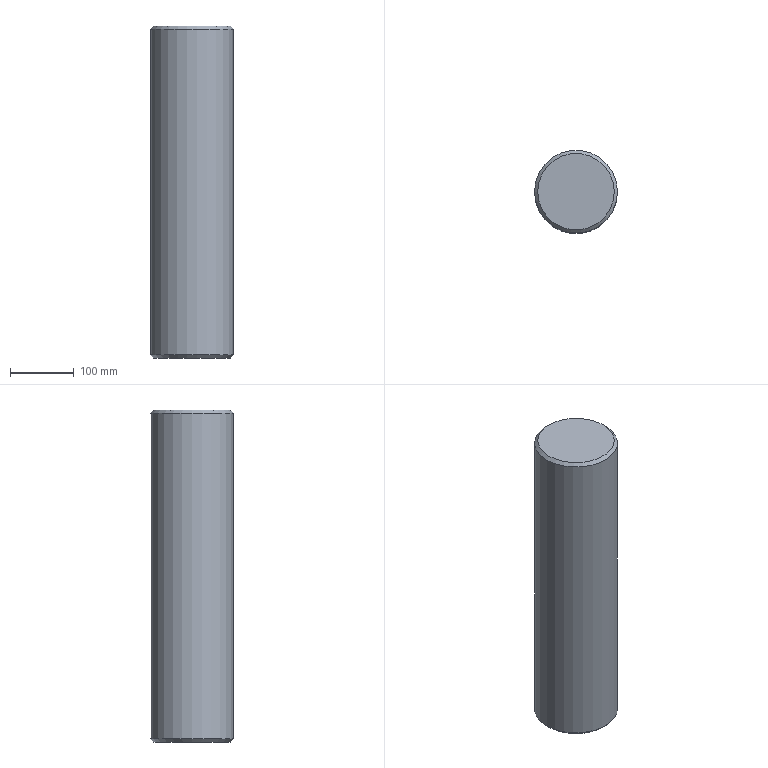Part | NX | features 顶梁掩护板柱销 2 | 1 solid | 5 faces | box 130 x 130 x 520 mm | volume 6892131 mm3 | plane 2 | cone 2 | cylinder 1 | commonest cylinder face diameters 130 x1
STEP:
#1=CARTESIAN_POINT('',(65.,0.,515.));
#2=VERTEX_POINT('',#1);
#3=CARTESIAN_POINT('',(0.,0.,515.));
#4=DIRECTION('',(0.,0.,1.));
#5=DIRECTION('',(1.,0.,0.));
#6=AXIS2_PLACEMENT_3D('',#3,#4,#5);
#7=CIRCLE('',#6,65.);
#8=EDGE_CURVE('',#2,#2,#7,.F.);
#9=ORIENTED_EDGE('',*,*,#8,.T.);
#10=EDGE_LOOP('',(#9));
#11=FACE_BOUND('',#10,.T.);
#12=CARTESIAN_POINT('',(65.,0.,5.));
#13=VERTEX_POINT('',#12);
#14=CARTESIAN_POINT('',(0.,0.,5.));
#15=DIRECTION('',(0.,0.,1.));
#16=DIRECTION('',(1.,0.,0.));
#17=AXIS2_PLACEMENT_3D('',#14,#15,#16);
#18=CIRCLE('',#17,65.);
#19=EDGE_CURVE('',#13,#13,#18,.T.);
#20=ORIENTED_EDGE('',*,*,#19,.T.);
#21=EDGE_LOOP('',(#20));
#22=FACE_BOUND('',#21,.T.);
#23=CARTESIAN_POINT('',(0.,0.,520.));
#24=DIRECTION('',(0.,0.,-1.));
#25=DIRECTION('',(-1.,0.,0.));
#26=AXIS2_PLACEMENT_3D('',#23,#24,#25);
#27=CYLINDRICAL_SURFACE('',#26,65.);
#28=ADVANCED_FACE('',(#11,#22),#27,.T.);
#29=CARTESIAN_POINT('',(60.,0.,520.));
#30=VERTEX_POINT('',#29);
#31=CARTESIAN_POINT('',(0.,0.,520.));
#32=DIRECTION('',(0.,0.,1.));
#33=DIRECTION('',(1.,0.,0.));
#34=AXIS2_PLACEMENT_3D('',#31,#32,#33);
#35=CIRCLE('',#34,60.);
#36=EDGE_CURVE('',#30,#30,#35,.T.);
#37=ORIENTED_EDGE('',*,*,#36,.T.);
#38=EDGE_LOOP('',(#37));
#39=FACE_BOUND('',#38,.T.);
#40=CARTESIAN_POINT('',(0.,0.,520.));
#41=DIRECTION('',(0.,0.,1.));
#42=DIRECTION('',(1.,0.,0.));
#43=AXIS2_PLACEMENT_3D('',#40,#41,#42);
#44=PLANE('',#43);
#45=ADVANCED_FACE('',(#39),#44,.T.);
#46=CARTESIAN_POINT('',(60.,0.,0.));
#47=VERTEX_POINT('',#46);
#48=CARTESIAN_POINT('',(0.,0.,0.));
#49=DIRECTION('',(0.,0.,1.));
#50=DIRECTION('',(1.,0.,0.));
#51=AXIS2_PLACEMENT_3D('',#48,#49,#50);
#52=CIRCLE('',#51,60.);
#53=EDGE_CURVE('',#47,#47,#52,.F.);
#54=ORIENTED_EDGE('',*,*,#53,.T.);
#55=EDGE_LOOP('',(#54));
#56=FACE_BOUND('',#55,.T.);
#57=CARTESIAN_POINT('',(0.,0.,0.));
#58=DIRECTION('',(0.,0.,1.));
#59=DIRECTION('',(1.,0.,0.));
#60=AXIS2_PLACEMENT_3D('',#57,#58,#59);
#61=PLANE('',#60);
#62=ADVANCED_FACE('',(#56),#61,.F.);
#63=ORIENTED_EDGE('',*,*,#8,.F.);
#64=EDGE_LOOP('',(#63));
#65=FACE_BOUND('',#64,.T.);
#66=ORIENTED_EDGE('',*,*,#36,.F.);
#67=EDGE_LOOP('',(#66));
#68=FACE_BOUND('',#67,.T.);
#69=CARTESIAN_POINT('',(0.,0.,520.));
#70=DIRECTION('',(0.,0.,-1.));
#71=DIRECTION('',(-1.,0.,0.));
#72=AXIS2_PLACEMENT_3D('',#69,#70,#71);
#73=CONICAL_SURFACE('',#72,60.,0.7854);
#74=ADVANCED_FACE('',(#65,#68),#73,.T.);
#75=ORIENTED_EDGE('',*,*,#53,.F.);
#76=EDGE_LOOP('',(#75));
#77=FACE_BOUND('',#76,.T.);
#78=ORIENTED_EDGE('',*,*,#19,.F.);
#79=EDGE_LOOP('',(#78));
#80=FACE_BOUND('',#79,.T.);
#81=CARTESIAN_POINT('',(0.,0.,5.));
#82=DIRECTION('',(0.,0.,1.));
#83=DIRECTION('',(1.,0.,0.));
#84=AXIS2_PLACEMENT_3D('',#81,#82,#83);
#85=CONICAL_SURFACE('',#84,65.,0.7854);
#86=ADVANCED_FACE('',(#77,#80),#85,.T.);
#87=CLOSED_SHELL('',(#28,#45,#62,#74,#86));
#88=MANIFOLD_SOLID_BREP('',#87);
#89=(LENGTH_UNIT()NAMED_UNIT(*)SI_UNIT(.MILLI.,.METRE.));
#90=UNCERTAINTY_MEASURE_WITH_UNIT(LENGTH_MEASURE(0.00001),#89,'','');
#91=(NAMED_UNIT(*)PLANE_ANGLE_UNIT()SI_UNIT($,.RADIAN.));
#92=(NAMED_UNIT(*)SI_UNIT($,.STERADIAN.)SOLID_ANGLE_UNIT());
#93=(GEOMETRIC_REPRESENTATION_CONTEXT(3)GLOBAL_UNCERTAINTY_ASSIGNED_CONTEXT((#90))GLOBAL_UNIT_ASSIGNED_CONTEXT((#89,#91,#92))REPRESENTATION_CONTEXT('',''));
#94=ADVANCED_BREP_SHAPE_REPRESENTATION('',(#88),#93);